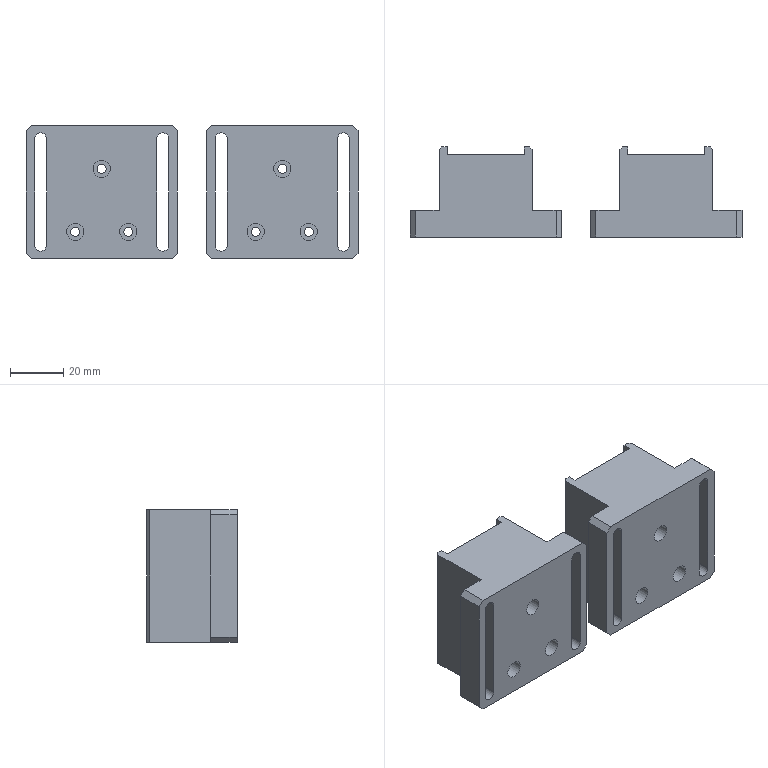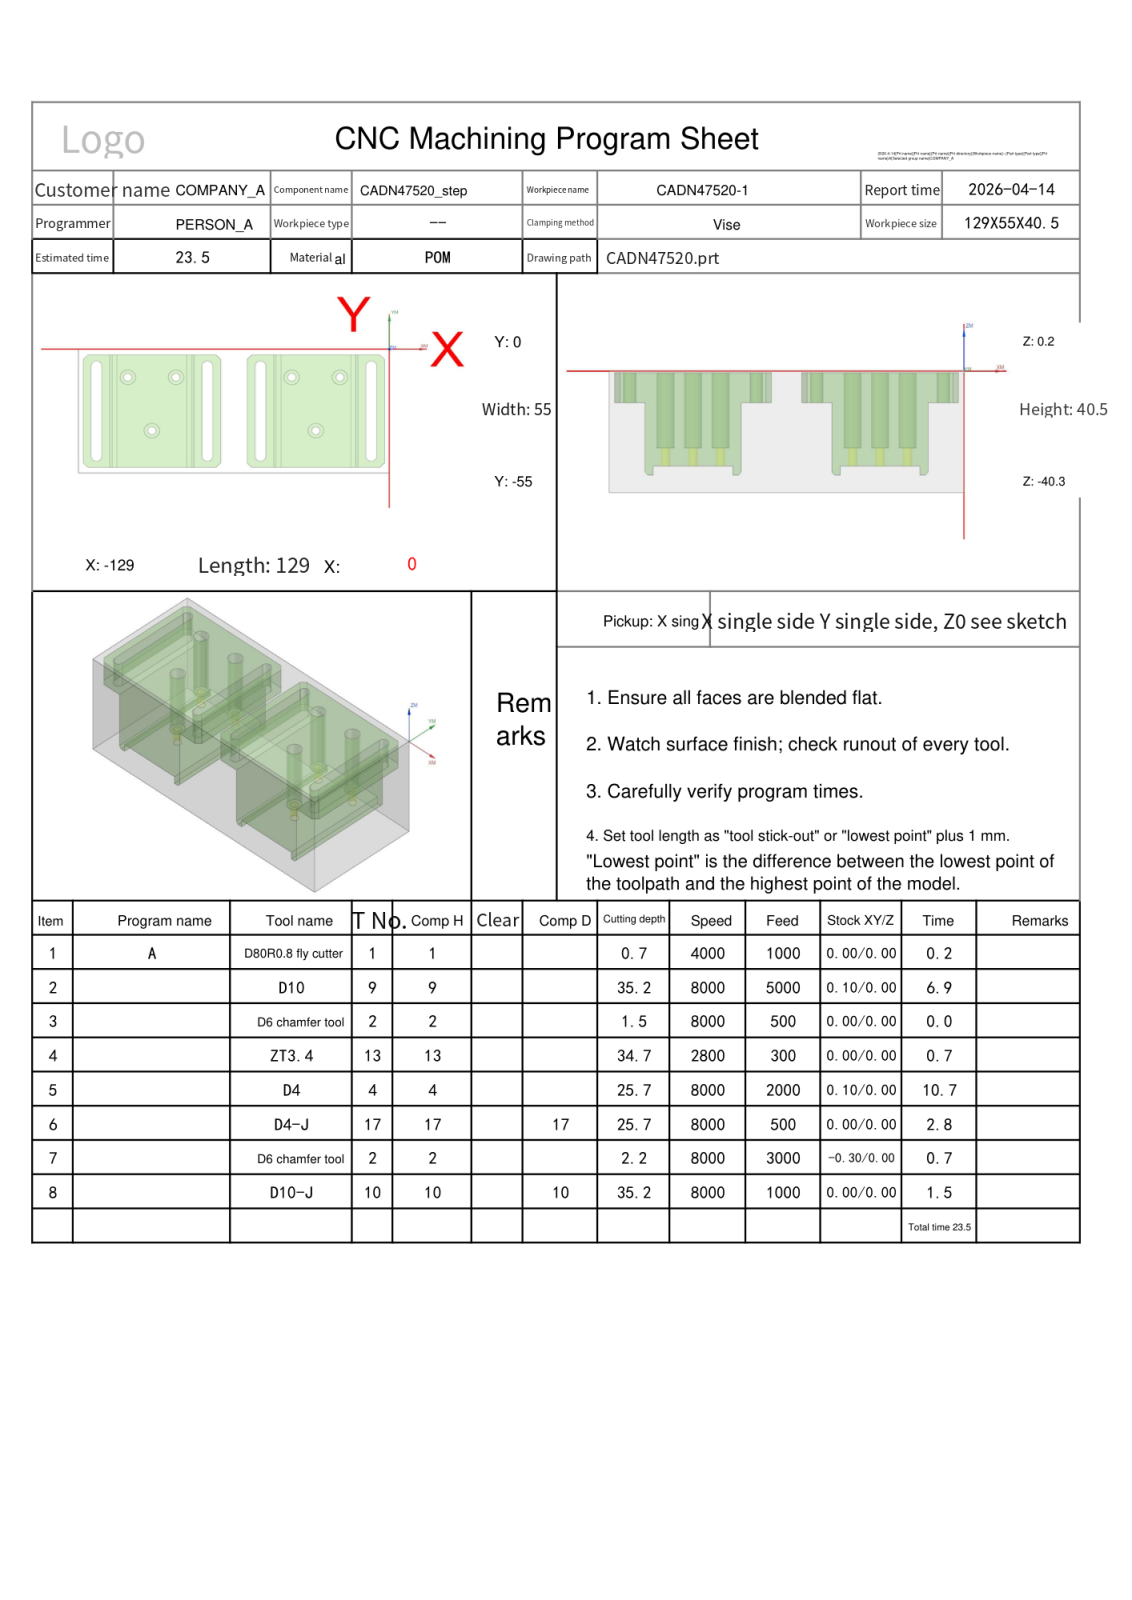NC program | NX | posted by the shop | part box 125 x 34 x 50 mm
Lines 34 to 772 of 5259:
N2 T09 M06
(D10  D=10. R=0. H=09 ce=0.10 di=0.00)
G00 G90 G54 X-98.5 Y-57.6 M03 S8000
G43 H09 Z19.5
M08
Z0.0
G01 X-125. Z-.055 F5000.
G02 X-128.606 Y-56.106 Z-.063 I0.0 J5.1
G01 X-130.606 Y-54.106 Z-.069
G02 X-132.1 Y-50.5 Z-.077 I3.606 J3.606
G01 Y-4.5 Z-.173
G02 X-130.606 Y-.894 Z-.181 I5.1 J0.0
G01 X-128.606 Y1.106 Z-.187
G02 X-125. Y2.6 Z-.195 I3.606 J-3.606
G01 X-72. Z-.305
G02 X-68.394 Y1.106 Z-.313 I0.0 J-5.1
G01 X-66.394 Y-.894 Z-.319
G02 X-64.9 Y-4.5 Z-.327 I-3.606 J-3.606
G01 Y-50.5 Z-.423
G02 X-66.394 Y-54.106 Z-.431 I-5.1 J0.0
G01 X-68.394 Y-56.106 Z-.437
G02 X-72. Y-57.6 Z-.445 I-3.606 J3.606
G01 X-125. Z-.555
G02 X-128.606 Y-56.106 Z-.563 I0.0 J5.1
G01 X-130.606 Y-54.106 Z-.569
G02 X-132.1 Y-50.5 Z-.577 I3.606 J3.606
G01 Y-4.5 Z-.673
G02 X-130.606 Y-.894 Z-.681 I5.1 J0.0
G01 X-128.606 Y1.106 Z-.687
G02 X-125. Y2.6 Z-.695 I3.606 J-3.606
G01 X-72. Z-.805
G02 X-68.394 Y1.106 Z-.813 I0.0 J-5.1
G01 X-66.394 Y-.894 Z-.819
G02 X-64.9 Y-4.5 Z-.827 I-3.606 J-3.606
G01 Y-50.5 Z-.923
G02 X-66.394 Y-54.106 Z-.931 I-5.1 J0.0
G01 X-68.394 Y-56.106 Z-.937
G02 X-72. Y-57.6 Z-.945 I-3.606 J3.606
G01 X-125. Z-1.055
G02 X-128.606 Y-56.106 Z-1.063 I0.0 J5.1
G01 X-130.606 Y-54.106 Z-1.069
G02 X-132.1 Y-50.5 Z-1.077 I3.606 J3.606
G01 Y-4.5 Z-1.173
G02 X-130.606 Y-.894 Z-1.181 I5.1 J0.0
G01 X-128.606 Y1.106 Z-1.187
G02 X-125. Y2.6 Z-1.195 I3.606 J-3.606
G01 X-72. Z-1.305
G02 X-68.394 Y1.106 Z-1.313 I0.0 J-5.1
G01 X-66.394 Y-.894 Z-1.319
G02 X-64.9 Y-4.5 Z-1.327 I-3.606 J-3.606
G01 Y-50.5 Z-1.423
G02 X-66.394 Y-54.106 Z-1.431 I-5.1 J0.0
G01 X-68.394 Y-56.106 Z-1.437
G02 X-72. Y-57.6 Z-1.445 I-3.606 J3.606
G01 X-125. Z-1.555
G02 X-128.606 Y-56.106 Z-1.563 I0.0 J5.1
G01 X-130.606 Y-54.106 Z-1.569
G02 X-132.1 Y-50.5 Z-1.577 I3.606 J3.606
G01 Y-4.5 Z-1.673
G02 X-130.606 Y-.894 Z-1.681 I5.1 J0.0
G01 X-128.606 Y1.106 Z-1.687
G02 X-125. Y2.6 Z-1.695 I3.606 J-3.606
G01 X-72. Z-1.805
G02 X-68.394 Y1.106 Z-1.813 I0.0 J-5.1
G01 X-66.394 Y-.894 Z-1.819
G02 X-64.9 Y-4.5 Z-1.827 I-3.606 J-3.606
G01 Y-50.5 Z-1.923
G02 X-66.394 Y-54.106 Z-1.931 I-5.1 J0.0
G01 X-68.394 Y-56.106 Z-1.937
G02 X-72. Y-57.6 Z-1.945 I-3.606 J3.606
G01 X-125. Z-2.055
G02 X-128.606 Y-56.106 Z-2.063 I0.0 J5.1
G01 X-130.606 Y-54.106 Z-2.069
G02 X-132.1 Y-50.5 Z-2.077 I3.606 J3.606
G01 Y-4.5 Z-2.173
G02 X-130.606 Y-.894 Z-2.181 I5.1 J0.0
G01 X-128.606 Y1.106 Z-2.187
G02 X-125. Y2.6 Z-2.195 I3.606 J-3.606
G01 X-72. Z-2.305
G02 X-68.394 Y1.106 Z-2.313 I0.0 J-5.1
G01 X-66.394 Y-.894 Z-2.319
G02 X-64.9 Y-4.5 Z-2.327 I-3.606 J-3.606
G01 Y-50.5 Z-2.423
G02 X-66.394 Y-54.106 Z-2.431 I-5.1 J0.0
G01 X-68.394 Y-56.106 Z-2.437
G02 X-72. Y-57.6 Z-2.445 I-3.606 J3.606
G01 X-125. Z-2.555
G02 X-128.606 Y-56.106 Z-2.563 I0.0 J5.1
G01 X-130.606 Y-54.106 Z-2.569
G02 X-132.1 Y-50.5 Z-2.577 I3.606 J3.606
G01 Y-4.5 Z-2.673
G02 X-130.606 Y-.894 Z-2.681 I5.1 J0.0
G01 X-128.606 Y1.106 Z-2.687
G02 X-125. Y2.6 Z-2.695 I3.606 J-3.606
G01 X-72. Z-2.805
G02 X-68.394 Y1.106 Z-2.813 I0.0 J-5.1
G01 X-66.394 Y-.894 Z-2.819
G02 X-64.9 Y-4.5 Z-2.827 I-3.606 J-3.606
G01 Y-50.5 Z-2.923
G02 X-66.394 Y-54.106 Z-2.931 I-5.1 J0.0
G01 X-68.394 Y-56.106 Z-2.937
G02 X-72. Y-57.6 Z-2.945 I-3.606 J3.606
G01 X-125. Z-3.055
G02 X-128.606 Y-56.106 Z-3.063 I0.0 J5.1
G01 X-130.606 Y-54.106 Z-3.069
G02 X-132.1 Y-50.5 Z-3.077 I3.606 J3.606
G01 Y-4.5 Z-3.173
G02 X-130.606 Y-.894 Z-3.181 I5.1 J0.0
G01 X-128.606 Y1.106 Z-3.187
G02 X-125. Y2.6 Z-3.195 I3.606 J-3.606
G01 X-72. Z-3.305
G02 X-68.394 Y1.106 Z-3.313 I0.0 J-5.1
G01 X-66.394 Y-.894 Z-3.319
G02 X-64.9 Y-4.5 Z-3.327 I-3.606 J-3.606
G01 Y-50.5 Z-3.423
G02 X-66.394 Y-54.106 Z-3.431 I-5.1 J0.0
G01 X-68.394 Y-56.106 Z-3.437
G02 X-72. Y-57.6 Z-3.445 I-3.606 J3.606
G01 X-125. Z-3.555
G02 X-128.606 Y-56.106 Z-3.563 I0.0 J5.1
G01 X-130.606 Y-54.106 Z-3.569
G02 X-132.1 Y-50.5 Z-3.577 I3.606 J3.606
G01 Y-4.5 Z-3.673
G02 X-130.606 Y-.894 Z-3.681 I5.1 J0.0
G01 X-128.606 Y1.106 Z-3.687
G02 X-125. Y2.6 Z-3.695 I3.606 J-3.606
G01 X-72. Z-3.805
G02 X-68.394 Y1.106 Z-3.813 I0.0 J-5.1
G01 X-66.394 Y-.894 Z-3.819
G02 X-64.9 Y-4.5 Z-3.827 I-3.606 J-3.606
G01 Y-50.5 Z-3.923
G02 X-66.394 Y-54.106 Z-3.931 I-5.1 J0.0
G01 X-68.394 Y-56.106 Z-3.937
G02 X-72. Y-57.6 Z-3.945 I-3.606 J3.606
G01 X-125. Z-4.055
G02 X-128.606 Y-56.106 Z-4.063 I0.0 J5.1
G01 X-130.606 Y-54.106 Z-4.069
G02 X-132.1 Y-50.5 Z-4.077 I3.606 J3.606
G01 Y-4.5 Z-4.173
G02 X-130.606 Y-.894 Z-4.181 I5.1 J0.0
G01 X-128.606 Y1.106 Z-4.187
G02 X-125. Y2.6 Z-4.195 I3.606 J-3.606
G01 X-72. Z-4.305
G02 X-68.394 Y1.106 Z-4.313 I0.0 J-5.1
G01 X-66.394 Y-.894 Z-4.319
G02 X-64.9 Y-4.5 Z-4.327 I-3.606 J-3.606
G01 Y-50.5 Z-4.423
G02 X-66.394 Y-54.106 Z-4.431 I-5.1 J0.0
G01 X-68.394 Y-56.106 Z-4.437
G02 X-72. Y-57.6 Z-4.445 I-3.606 J3.606
G01 X-125. Z-4.555
G02 X-128.606 Y-56.106 Z-4.563 I0.0 J5.1
G01 X-130.606 Y-54.106 Z-4.569
G02 X-132.1 Y-50.5 Z-4.577 I3.606 J3.606
G01 Y-4.5 Z-4.673
G02 X-130.606 Y-.894 Z-4.681 I5.1 J0.0
G01 X-128.606 Y1.106 Z-4.687
G02 X-125. Y2.6 Z-4.695 I3.606 J-3.606
G01 X-72. Z-4.805
G02 X-68.394 Y1.106 Z-4.813 I0.0 J-5.1
G01 X-66.394 Y-.894 Z-4.819
G02 X-64.9 Y-4.5 Z-4.827 I-3.606 J-3.606
G01 Y-50.5 Z-4.923
G02 X-66.394 Y-54.106 Z-4.931 I-5.1 J0.0
G01 X-68.394 Y-56.106 Z-4.937
G02 X-72. Y-57.6 Z-4.945 I-3.606 J3.606
G01 X-125. Z-5.055
G02 X-128.606 Y-56.106 Z-5.063 I0.0 J5.1
G01 X-130.606 Y-54.106 Z-5.069
G02 X-132.1 Y-50.5 Z-5.077 I3.606 J3.606
G01 Y-4.5 Z-5.173
G02 X-130.606 Y-.894 Z-5.181 I5.1 J0.0
G01 X-128.606 Y1.106 Z-5.187
G02 X-125. Y2.6 Z-5.195 I3.606 J-3.606
G01 X-72. Z-5.305
G02 X-68.394 Y1.106 Z-5.313 I0.0 J-5.1
G01 X-66.394 Y-.894 Z-5.319
G02 X-64.9 Y-4.5 Z-5.327 I-3.606 J-3.606
G01 Y-50.5 Z-5.423
G02 X-66.394 Y-54.106 Z-5.431 I-5.1 J0.0
G01 X-68.394 Y-56.106 Z-5.437
G02 X-72. Y-57.6 Z-5.445 I-3.606 J3.606
G01 X-125. Z-5.555
G02 X-128.606 Y-56.106 Z-5.563 I0.0 J5.1
G01 X-130.606 Y-54.106 Z-5.569
G02 X-132.1 Y-50.5 Z-5.577 I3.606 J3.606
G01 Y-4.5 Z-5.673
G02 X-130.606 Y-.894 Z-5.681 I5.1 J0.0
G01 X-128.606 Y1.106 Z-5.687
G02 X-125. Y2.6 Z-5.695 I3.606 J-3.606
G01 X-72. Z-5.805
G02 X-68.394 Y1.106 Z-5.813 I0.0 J-5.1
G01 X-66.394 Y-.894 Z-5.819
G02 X-64.9 Y-4.5 Z-5.827 I-3.606 J-3.606
G01 Y-50.5 Z-5.923
G02 X-66.394 Y-54.106 Z-5.931 I-5.1 J0.0
G01 X-68.394 Y-56.106 Z-5.937
G02 X-72. Y-57.6 Z-5.945 I-3.606 J3.606
G01 X-125. Z-6.055
G02 X-128.606 Y-56.106 Z-6.063 I0.0 J5.1
G01 X-130.606 Y-54.106 Z-6.069
G02 X-132.1 Y-50.5 Z-6.077 I3.606 J3.606
G01 Y-4.5 Z-6.173
G02 X-130.606 Y-.894 Z-6.181 I5.1 J0.0
G01 X-128.606 Y1.106 Z-6.187
G02 X-125. Y2.6 Z-6.195 I3.606 J-3.606
G01 X-72. Z-6.305
G02 X-68.394 Y1.106 Z-6.313 I0.0 J-5.1
G01 X-66.394 Y-.894 Z-6.319
G02 X-64.9 Y-4.5 Z-6.327 I-3.606 J-3.606
G01 Y-50.5 Z-6.423
G02 X-66.394 Y-54.106 Z-6.431 I-5.1 J0.0
G01 X-68.394 Y-56.106 Z-6.437
G02 X-72. Y-57.6 Z-6.445 I-3.606 J3.606
G01 X-125. Z-6.555
G02 X-128.606 Y-56.106 Z-6.563 I0.0 J5.1
G01 X-130.606 Y-54.106 Z-6.569
G02 X-132.1 Y-50.5 Z-6.577 I3.606 J3.606
G01 Y-4.5 Z-6.673
G02 X-130.606 Y-.894 Z-6.681 I5.1 J0.0
G01 X-128.606 Y1.106 Z-6.687
G02 X-125. Y2.6 Z-6.695 I3.606 J-3.606
G01 X-72. Z-6.805
G02 X-68.394 Y1.106 Z-6.813 I0.0 J-5.1
G01 X-66.394 Y-.894 Z-6.819
G02 X-64.9 Y-4.5 Z-6.827 I-3.606 J-3.606
G01 Y-50.5 Z-6.923
G02 X-66.394 Y-54.106 Z-6.931 I-5.1 J0.0
G01 X-68.394 Y-56.106 Z-6.937
G02 X-72. Y-57.6 Z-6.945 I-3.606 J3.606
G01 X-125. Z-7.055
G02 X-128.606 Y-56.106 Z-7.063 I0.0 J5.1
G01 X-130.606 Y-54.106 Z-7.069
G02 X-132.1 Y-50.5 Z-7.077 I3.606 J3.606
G01 Y-4.5 Z-7.173
G02 X-130.606 Y-.894 Z-7.181 I5.1 J0.0
G01 X-128.606 Y1.106 Z-7.187
G02 X-125. Y2.6 Z-7.195 I3.606 J-3.606
G01 X-72. Z-7.305
G02 X-68.394 Y1.106 Z-7.313 I0.0 J-5.1
G01 X-66.394 Y-.894 Z-7.319
G02 X-64.9 Y-4.5 Z-7.327 I-3.606 J-3.606
G01 Y-50.5 Z-7.423
G02 X-66.394 Y-54.106 Z-7.431 I-5.1 J0.0
G01 X-68.394 Y-56.106 Z-7.437
G02 X-72. Y-57.6 Z-7.445 I-3.606 J3.606
G01 X-125. Z-7.555
G02 X-128.606 Y-56.106 Z-7.563 I0.0 J5.1
G01 X-130.606 Y-54.106 Z-7.569
G02 X-132.1 Y-50.5 Z-7.577 I3.606 J3.606
G01 Y-4.5 Z-7.673
G02 X-130.606 Y-.894 Z-7.681 I5.1 J0.0
G01 X-128.606 Y1.106 Z-7.687
G02 X-125. Y2.6 Z-7.695 I3.606 J-3.606
G01 X-72. Z-7.805
G02 X-68.394 Y1.106 Z-7.813 I0.0 J-5.1
G01 X-66.394 Y-.894 Z-7.819
G02 X-64.9 Y-4.5 Z-7.827 I-3.606 J-3.606
G01 Y-50.5 Z-7.923
G02 X-66.394 Y-54.106 Z-7.931 I-5.1 J0.0
G01 X-68.394 Y-56.106 Z-7.937
G02 X-72. Y-57.6 Z-7.945 I-3.606 J3.606
G01 X-125. Z-8.055
G02 X-128.606 Y-56.106 Z-8.063 I0.0 J5.1
G01 X-130.606 Y-54.106 Z-8.069
G02 X-132.1 Y-50.5 Z-8.077 I3.606 J3.606
G01 Y-4.5 Z-8.173
G02 X-130.606 Y-.894 Z-8.181 I5.1 J0.0
G01 X-128.606 Y1.106 Z-8.187
G02 X-125. Y2.6 Z-8.195 I3.606 J-3.606
G01 X-72. Z-8.305
G02 X-68.394 Y1.106 Z-8.313 I0.0 J-5.1
G01 X-66.394 Y-.894 Z-8.319
G02 X-64.9 Y-4.5 Z-8.327 I-3.606 J-3.606
G01 Y-50.5 Z-8.423
G02 X-66.394 Y-54.106 Z-8.431 I-5.1 J0.0
G01 X-68.394 Y-56.106 Z-8.437
G02 X-72. Y-57.6 Z-8.445 I-3.606 J3.606
G01 X-125. Z-8.555
G02 X-128.606 Y-56.106 Z-8.563 I0.0 J5.1
G01 X-130.606 Y-54.106 Z-8.569
G02 X-132.1 Y-50.5 Z-8.577 I3.606 J3.606
G01 Y-4.5 Z-8.673
G02 X-130.606 Y-.894 Z-8.681 I5.1 J0.0
G01 X-128.606 Y1.106 Z-8.687
G02 X-125. Y2.6 Z-8.695 I3.606 J-3.606
G01 X-72. Z-8.805
G02 X-68.394 Y1.106 Z-8.813 I0.0 J-5.1
G01 X-66.394 Y-.894 Z-8.819
G02 X-64.9 Y-4.5 Z-8.827 I-3.606 J-3.606
G01 Y-50.5 Z-8.923
G02 X-66.394 Y-54.106 Z-8.931 I-5.1 J0.0
G01 X-68.394 Y-56.106 Z-8.937
G02 X-72. Y-57.6 Z-8.945 I-3.606 J3.606
G01 X-125. Z-9.055
G02 X-128.606 Y-56.106 Z-9.063 I0.0 J5.1
G01 X-130.606 Y-54.106 Z-9.069
G02 X-132.1 Y-50.5 Z-9.077 I3.606 J3.606
G01 Y-4.5 Z-9.173
G02 X-130.606 Y-.894 Z-9.181 I5.1 J0.0
G01 X-128.606 Y1.106 Z-9.187
G02 X-125. Y2.6 Z-9.195 I3.606 J-3.606
G01 X-72. Z-9.305
G02 X-68.394 Y1.106 Z-9.313 I0.0 J-5.1
G01 X-66.394 Y-.894 Z-9.319
G02 X-64.9 Y-4.5 Z-9.327 I-3.606 J-3.606
G01 Y-50.5 Z-9.423
G02 X-66.394 Y-54.106 Z-9.431 I-5.1 J0.0
G01 X-68.394 Y-56.106 Z-9.437
G02 X-72. Y-57.6 Z-9.445 I-3.606 J3.606
G01 X-125. Z-9.555
G02 X-128.606 Y-56.106 Z-9.563 I0.0 J5.1
G01 X-130.606 Y-54.106 Z-9.569
G02 X-132.1 Y-50.5 Z-9.577 I3.606 J3.606
G01 Y-4.5 Z-9.673
G02 X-130.606 Y-.894 Z-9.681 I5.1 J0.0
G01 X-128.606 Y1.106 Z-9.687
G02 X-125. Y2.6 Z-9.695 I3.606 J-3.606
G01 X-72. Z-9.805
G02 X-68.394 Y1.106 Z-9.813 I0.0 J-5.1
G01 X-66.394 Y-.894 Z-9.819
G02 X-64.9 Y-4.5 Z-9.827 I-3.606 J-3.606
G01 Y-50.5 Z-9.923
G02 X-66.394 Y-54.106 Z-9.931 I-5.1 J0.0
G01 X-68.394 Y-56.106 Z-9.937
G02 X-72. Y-57.6 Z-9.945 I-3.606 J3.606
G01 X-125. Z-10.055
G02 X-128.606 Y-56.106 Z-10.063 I0.0 J5.1
G01 X-130.606 Y-54.106 Z-10.069
G02 X-132.1 Y-50.5 Z-10.077 I3.606 J3.606
G01 Y-4.5 Z-10.173
G02 X-130.606 Y-.894 Z-10.181 I5.1 J0.0
G01 X-128.606 Y1.106 Z-10.187
G02 X-125. Y2.6 Z-10.195 I3.606 J-3.606
G01 X-72. Z-10.305
G02 X-68.394 Y1.106 Z-10.313 I0.0 J-5.1
G01 X-66.394 Y-.894 Z-10.319
G02 X-64.9 Y-4.5 Z-10.327 I-3.606 J-3.606
G01 Y-50.5 Z-10.423
G02 X-66.394 Y-54.106 Z-10.431 I-5.1 J0.0
G01 X-68.394 Y-56.106 Z-10.437
G02 X-72. Y-57.6 Z-10.445 I-3.606 J3.606
G01 X-125. Z-10.555
G02 X-128.606 Y-56.106 Z-10.563 I0.0 J5.1
G01 X-130.606 Y-54.106 Z-10.569
G02 X-132.1 Y-50.5 Z-10.577 I3.606 J3.606
G01 Y-4.5 Z-10.673
G02 X-130.606 Y-.894 Z-10.681 I5.1 J0.0
G01 X-128.606 Y1.106 Z-10.687
G02 X-125. Y2.6 Z-10.695 I3.606 J-3.606
G01 X-72. Z-10.805
G02 X-68.394 Y1.106 Z-10.813 I0.0 J-5.1
G01 X-66.394 Y-.894 Z-10.819
G02 X-64.9 Y-4.5 Z-10.827 I-3.606 J-3.606
G01 Y-50.5 Z-10.923
G02 X-66.394 Y-54.106 Z-10.931 I-5.1 J0.0
G01 X-68.394 Y-56.106 Z-10.937
G02 X-72. Y-57.6 Z-10.945 I-3.606 J3.606
G01 X-125. Z-11.055
G02 X-128.606 Y-56.106 Z-11.063 I0.0 J5.1
G01 X-130.606 Y-54.106 Z-11.069
G02 X-132.1 Y-50.5 Z-11.077 I3.606 J3.606
G01 Y-4.5 Z-11.173
G02 X-130.606 Y-.894 Z-11.181 I5.1 J0.0
G01 X-128.606 Y1.106 Z-11.187
G02 X-125. Y2.6 Z-11.195 I3.606 J-3.606
G01 X-72. Z-11.305
G02 X-68.394 Y1.106 Z-11.313 I0.0 J-5.1
G01 X-66.394 Y-.894 Z-11.319
G02 X-64.9 Y-4.5 Z-11.327 I-3.606 J-3.606
G01 Y-50.5 Z-11.423
G02 X-66.394 Y-54.106 Z-11.431 I-5.1 J0.0
G01 X-68.394 Y-56.106 Z-11.437
G02 X-72. Y-57.6 Z-11.445 I-3.606 J3.606
G01 X-125. Z-11.555
G02 X-128.606 Y-56.106 Z-11.563 I0.0 J5.1
G01 X-130.606 Y-54.106 Z-11.569
G02 X-132.1 Y-50.5 Z-11.577 I3.606 J3.606
G01 Y-4.5 Z-11.673
G02 X-130.606 Y-.894 Z-11.681 I5.1 J0.0
G01 X-128.606 Y1.106 Z-11.687
G02 X-125. Y2.6 Z-11.695 I3.606 J-3.606
G01 X-72. Z-11.805
G02 X-68.394 Y1.106 Z-11.813 I0.0 J-5.1
G01 X-66.394 Y-.894 Z-11.819
G02 X-64.9 Y-4.5 Z-11.827 I-3.606 J-3.606
G01 Y-50.5 Z-11.923
G02 X-66.394 Y-54.106 Z-11.931 I-5.1 J0.0
G01 X-68.394 Y-56.106 Z-11.937
G02 X-72. Y-57.6 Z-11.945 I-3.606 J3.606
G01 X-125. Z-12.055
G02 X-128.606 Y-56.106 Z-12.063 I0.0 J5.1
G01 X-130.606 Y-54.106 Z-12.069
G02 X-132.1 Y-50.5 Z-12.077 I3.606 J3.606
G01 Y-4.5 Z-12.173
G02 X-130.606 Y-.894 Z-12.181 I5.1 J0.0
G01 X-128.606 Y1.106 Z-12.187
G02 X-125. Y2.6 Z-12.195 I3.606 J-3.606
G01 X-72. Z-12.305
G02 X-68.394 Y1.106 Z-12.313 I0.0 J-5.1
G01 X-66.394 Y-.894 Z-12.319
G02 X-64.9 Y-4.5 Z-12.327 I-3.606 J-3.606
G01 Y-50.5 Z-12.423
G02 X-66.394 Y-54.106 Z-12.431 I-5.1 J0.0
G01 X-68.394 Y-56.106 Z-12.437
G02 X-72. Y-57.6 Z-12.445 I-3.606 J3.606
G01 X-125. Z-12.555
G02 X-128.606 Y-56.106 Z-12.563 I0.0 J5.1
G01 X-130.606 Y-54.106 Z-12.569
G02 X-132.1 Y-50.5 Z-12.577 I3.606 J3.606
G01 Y-4.5 Z-12.673
G02 X-130.606 Y-.894 Z-12.681 I5.1 J0.0
G01 X-128.606 Y1.106 Z-12.687
G02 X-125. Y2.6 Z-12.695 I3.606 J-3.606
G01 X-72. Z-12.805
G02 X-68.394 Y1.106 Z-12.813 I0.0 J-5.1
G01 X-66.394 Y-.894 Z-12.819
G02 X-64.9 Y-4.5 Z-12.827 I-3.606 J-3.606
G01 Y-50.5 Z-12.923
G02 X-66.394 Y-54.106 Z-12.931 I-5.1 J0.0
G01 X-68.394 Y-56.106 Z-12.937
G02 X-72. Y-57.6 Z-12.945 I-3.606 J3.606
G01 X-125. Z-13.055
G02 X-128.606 Y-56.106 Z-13.063 I0.0 J5.1
G01 X-130.606 Y-54.106 Z-13.069
G02 X-132.1 Y-50.5 Z-13.077 I3.606 J3.606
G01 Y-4.5 Z-13.173
G02 X-130.606 Y-.894 Z-13.181 I5.1 J0.0
G01 X-128.606 Y1.106 Z-13.187
G02 X-125. Y2.6 Z-13.195 I3.606 J-3.606
G01 X-72. Z-13.305
G02 X-68.394 Y1.106 Z-13.313 I0.0 J-5.1
G01 X-66.394 Y-.894 Z-13.319
G02 X-64.9 Y-4.5 Z-13.327 I-3.606 J-3.606
G01 Y-50.5 Z-13.423
G02 X-66.394 Y-54.106 Z-13.431 I-5.1 J0.0
G01 X-68.394 Y-56.106 Z-13.437
G02 X-72. Y-57.6 Z-13.445 I-3.606 J3.606
G01 X-125. Z-13.555
G02 X-128.606 Y-56.106 Z-13.563 I0.0 J5.1
G01 X-130.606 Y-54.106 Z-13.569
G02 X-132.1 Y-50.5 Z-13.577 I3.606 J3.606
G01 Y-4.5 Z-13.673
G02 X-130.606 Y-.894 Z-13.681 I5.1 J0.0
G01 X-128.606 Y1.106 Z-13.687
G02 X-125. Y2.6 Z-13.695 I3.606 J-3.606
G01 X-72. Z-13.805
G02 X-68.394 Y1.106 Z-13.813 I0.0 J-5.1
G01 X-66.394 Y-.894 Z-13.819
G02 X-64.9 Y-4.5 Z-13.827 I-3.606 J-3.606
G01 Y-50.5 Z-13.923
G02 X-66.394 Y-54.106 Z-13.931 I-5.1 J0.0
G01 X-68.394 Y-56.106 Z-13.937
G02 X-72. Y-57.6 Z-13.945 I-3.606 J3.606
G01 X-125. Z-14.055
G02 X-128.606 Y-56.106 Z-14.063 I0.0 J5.1
G01 X-130.606 Y-54.106 Z-14.069
G02 X-132.1 Y-50.5 Z-14.077 I3.606 J3.606
G01 Y-4.5 Z-14.173
G02 X-130.606 Y-.894 Z-14.181 I5.1 J0.0
G01 X-128.606 Y1.106 Z-14.187
G02 X-125. Y2.6 Z-14.195 I3.606 J-3.606
G01 X-72. Z-14.305
G02 X-68.394 Y1.106 Z-14.313 I0.0 J-5.1
G01 X-66.394 Y-.894 Z-14.319
G02 X-64.9 Y-4.5 Z-14.327 I-3.606 J-3.606
G01 Y-50.5 Z-14.423
G02 X-66.394 Y-54.106 Z-14.431 I-5.1 J0.0
G01 X-68.394 Y-56.106 Z-14.437
G02 X-72. Y-57.6 Z-14.445 I-3.606 J3.606
G01 X-125. Z-14.555
G02 X-128.606 Y-56.106 Z-14.563 I0.0 J5.1
G01 X-130.606 Y-54.106 Z-14.569
G02 X-132.1 Y-50.5 Z-14.577 I3.606 J3.606
G01 Y-4.5 Z-14.673
G02 X-130.606 Y-.894 Z-14.681 I5.1 J0.0
G01 X-128.606 Y1.106 Z-14.687
G02 X-125. Y2.6 Z-14.695 I3.606 J-3.606
G01 X-72. Z-14.805
G02 X-68.394 Y1.106 Z-14.813 I0.0 J-5.1
G01 X-66.394 Y-.894 Z-14.819
G02 X-64.9 Y-4.5 Z-14.827 I-3.606 J-3.606
G01 Y-50.5 Z-14.923
G02 X-66.394 Y-54.106 Z-14.931 I-5.1 J0.0
G01 X-68.394 Y-56.106 Z-14.937
G02 X-72. Y-57.6 Z-14.945 I-3.606 J3.606
G01 X-125. Z-15.055
G02 X-128.606 Y-56.106 Z-15.063 I0.0 J5.1
G01 X-130.606 Y-54.106 Z-15.069
G02 X-132.1 Y-50.5 Z-15.077 I3.606 J3.606
G01 Y-4.5 Z-15.173
G02 X-130.606 Y-.894 Z-15.181 I5.1 J0.0
G01 X-128.606 Y1.106 Z-15.187
G02 X-125. Y2.6 Z-15.195 I3.606 J-3.606
G01 X-72. Z-15.305
G02 X-68.394 Y1.106 Z-15.313 I0.0 J-5.1
G01 X-66.394 Y-.894 Z-15.319
G02 X-64.9 Y-4.5 Z-15.327 I-3.606 J-3.606
G01 Y-50.5 Z-15.423
G02 X-66.394 Y-54.106 Z-15.431 I-5.1 J0.0
G01 X-68.394 Y-56.106 Z-15.437
G02 X-72. Y-57.6 Z-15.445 I-3.606 J3.606
G01 X-125. Z-15.555
G02 X-128.606 Y-56.106 Z-15.563 I0.0 J5.1
G01 X-130.606 Y-54.106 Z-15.569
G02 X-132.1 Y-50.5 Z-15.577 I3.606 J3.606
G01 Y-4.5 Z-15.673
G02 X-130.606 Y-.894 Z-15.681 I5.1 J0.0
G01 X-128.606 Y1.106 Z-15.687
G02 X-125. Y2.6 Z-15.695 I3.606 J-3.606
G01 X-72. Z-15.805
G02 X-68.394 Y1.106 Z-15.813 I0.0 J-5.1
G01 X-66.394 Y-.894 Z-15.819
G02 X-64.9 Y-4.5 Z-15.827 I-3.606 J-3.606
G01 Y-50.5 Z-15.923
G02 X-66.394 Y-54.106 Z-15.931 I-5.1 J0.0
G01 X-68.394 Y-56.106 Z-15.937
G02 X-72. Y-57.6 Z-15.945 I-3.606 J3.606
G01 X-125. Z-16.055
G02 X-128.606 Y-56.106 Z-16.063 I0.0 J5.1
G01 X-130.606 Y-54.106 Z-16.069
G02 X-132.1 Y-50.5 Z-16.077 I3.606 J3.606
G01 Y-4.5 Z-16.173
G02 X-130.606 Y-.894 Z-16.181 I5.1 J0.0
G01 X-128.606 Y1.106 Z-16.187
G02 X-125. Y2.6 Z-16.195 I3.606 J-3.606
G01 X-72. Z-16.305
G02 X-68.394 Y1.106 Z-16.313 I0.0 J-5.1
G01 X-66.394 Y-.894 Z-16.319
G02 X-64.9 Y-4.5 Z-16.327 I-3.606 J-3.606
G01 Y-50.5 Z-16.423
G02 X-66.394 Y-54.106 Z-16.431 I-5.1 J0.0
G01 X-68.394 Y-56.106 Z-16.437
G02 X-72. Y-57.6 Z-16.445 I-3.606 J3.606
G01 X-125. Z-16.555
G02 X-128.606 Y-56.106 Z-16.563 I0.0 J5.1
G01 X-130.606 Y-54.106 Z-16.569
G02 X-132.1 Y-50.5 Z-16.577 I3.606 J3.606
G01 Y-4.5 Z-16.673
G02 X-130.606 Y-.894 Z-16.681 I5.1 J0.0
G01 X-128.606 Y1.106 Z-16.687
G02 X-125. Y2.6 Z-16.695 I3.606 J-3.606
G01 X-72. Z-16.805
G02 X-68.394 Y1.106 Z-16.813 I0.0 J-5.1
G01 X-66.394 Y-.894 Z-16.819
G02 X-64.9 Y-4.5 Z-16.827 I-3.606 J-3.606
G01 Y-50.5 Z-16.923
G02 X-66.394 Y-54.106 Z-16.931 I-5.1 J0.0
G01 X-68.394 Y-56.106 Z-16.937
G02 X-72. Y-57.6 Z-16.945 I-3.606 J3.606
G01 X-125. Z-17.055
G02 X-128.606 Y-56.106 Z-17.063 I0.0 J5.1
G01 X-130.606 Y-54.106 Z-17.069
G02 X-132.1 Y-50.5 Z-17.077 I3.606 J3.606
G01 Y-4.5 Z-17.173
G02 X-130.606 Y-.894 Z-17.181 I5.1 J0.0
G01 X-128.606 Y1.106 Z-17.187
G02 X-125. Y2.6 Z-17.195 I3.606 J-3.606
G01 X-72. Z-17.305
G02 X-68.394 Y1.106 Z-17.313 I0.0 J-5.1
G01 X-66.394 Y-.894 Z-17.319
G02 X-64.9 Y-4.5 Z-17.327 I-3.606 J-3.606
G01 Y-50.5 Z-17.423
G02 X-66.394 Y-54.106 Z-17.431 I-5.1 J0.0
G01 X-68.394 Y-56.106 Z-17.437
G02 X-72. Y-57.6 Z-17.445 I-3.606 J3.606
G01 X-125. Z-17.555
G02 X-128.606 Y-56.106 Z-17.563 I0.0 J5.1
G01 X-130.606 Y-54.106 Z-17.569
G02 X-132.1 Y-50.5 Z-17.577 I3.606 J3.606
G01 Y-4.5 Z-17.673
G02 X-130.606 Y-.894 Z-17.681 I5.1 J0.0
G01 X-128.606 Y1.106 Z-17.687
G02 X-125. Y2.6 Z-17.695 I3.606 J-3.606
G01 X-72. Z-17.805
G02 X-68.394 Y1.106 Z-17.813 I0.0 J-5.1
G01 X-66.394 Y-.894 Z-17.819
G02 X-64.9 Y-4.5 Z-17.827 I-3.606 J-3.606
G01 Y-50.5 Z-17.923
G02 X-66.394 Y-54.106 Z-17.931 I-5.1 J0.0
G01 X-68.394 Y-56.106 Z-17.937
G02 X-72. Y-57.6 Z-17.945 I-3.606 J3.606
G01 X-125. Z-18.055
G02 X-128.606 Y-56.106 Z-18.063 I0.0 J5.1
G01 X-130.606 Y-54.106 Z-18.069
G02 X-132.1 Y-50.5 Z-18.077 I3.606 J3.606
G01 Y-4.5 Z-18.173
G02 X-130.606 Y-.894 Z-18.181 I5.1 J0.0
G01 X-128.606 Y1.106 Z-18.187
G02 X-125. Y2.6 Z-18.195 I3.606 J-3.606
G01 X-72. Z-18.305
G02 X-68.394 Y1.106 Z-18.313 I0.0 J-5.1
G01 X-66.394 Y-.894 Z-18.319
G02 X-64.9 Y-4.5 Z-18.327 I-3.606 J-3.606
G01 Y-50.5 Z-18.423
G02 X-66.394 Y-54.106 Z-18.431 I-5.1 J0.0
G01 X-68.394 Y-56.106 Z-18.437
G02 X-72. Y-57.6 Z-18.445 I-3.606 J3.606
G01 X-125. Z-18.555
G02 X-128.606 Y-56.106 Z-18.563 I0.0 J5.1
G01 X-130.606 Y-54.106 Z-18.569
G02 X-132.1 Y-50.5 Z-18.577 I3.606 J3.606
G01 Y-4.5 Z-18.673
G02 X-130.606 Y-.894 Z-18.681 I5.1 J0.0
G01 X-128.606 Y1.106 Z-18.687
G02 X-125. Y2.6 Z-18.695 I3.606 J-3.606
G01 X-72. Z-18.805
G02 X-68.394 Y1.106 Z-18.813 I0.0 J-5.1
G01 X-66.394 Y-.894 Z-18.819
G02 X-64.9 Y-4.5 Z-18.827 I-3.606 J-3.606
G01 Y-50.5 Z-18.923
G02 X-66.394 Y-54.106 Z-18.931 I-5.1 J0.0
G01 X-68.394 Y-56.106 Z-18.937
G02 X-72. Y-57.6 Z-18.945 I-3.606 J3.606
G01 X-125. Z-19.055
G02 X-128.606 Y-56.106 Z-19.063 I0.0 J5.1
G01 X-130.606 Y-54.106 Z-19.069
G02 X-132.1 Y-50.5 Z-19.077 I3.606 J3.606
G01 Y-4.5 Z-19.173
G02 X-130.606 Y-.894 Z-19.181 I5.1 J0.0
G01 X-128.606 Y1.106 Z-19.187
G02 X-125. Y2.6 Z-19.195 I3.606 J-3.606
G01 X-72. Z-19.305
G02 X-68.394 Y1.106 Z-19.313 I0.0 J-5.1
G01 X-66.394 Y-.894 Z-19.319
G02 X-64.9 Y-4.5 Z-19.327 I-3.606 J-3.606
G01 Y-50.5 Z-19.423
G02 X-66.394 Y-54.106 Z-19.431 I-5.1 J0.0
G01 X-68.394 Y-56.106 Z-19.437
G02 X-72. Y-57.6 Z-19.445 I-3.606 J3.606
G01 X-125. Z-19.555
G02 X-128.606 Y-56.106 Z-19.563 I0.0 J5.1
G01 X-130.606 Y-54.106 Z-19.569
G02 X-132.1 Y-50.5 Z-19.577 I3.606 J3.606
G01 Y-4.5 Z-19.673
G02 X-130.606 Y-.894 Z-19.681 I5.1 J0.0
G01 X-128.606 Y1.106 Z-19.687
G02 X-125. Y2.6 Z-19.695 I3.606 J-3.606
G01 X-72. Z-19.805
G02 X-68.394 Y1.106 Z-19.813 I0.0 J-5.1
G01 X-66.394 Y-.894 Z-19.819
G02 X-64.9 Y-4.5 Z-19.827 I-3.606 J-3.606
G01 Y-50.5 Z-19.923
G02 X-66.394 Y-54.106 Z-19.931 I-5.1 J0.0
G01 X-68.394 Y-56.106 Z-19.937
G02 X-72. Y-57.6 Z-19.945 I-3.606 J3.606
G01 X-125. Z-20.055
G02 X-128.606 Y-56.106 Z-20.063 I0.0 J5.1
G01 X-130.606 Y-54.106 Z-20.069
G02 X-132.1 Y-50.5 Z-20.077 I3.606 J3.606
G01 Y-4.5 Z-20.173
G02 X-130.606 Y-.894 Z-20.181 I5.1 J0.0
G01 X-128.606 Y1.106 Z-20.187
G02 X-125. Y2.6 Z-20.195 I3.606 J-3.606
G01 X-72. Z-20.305
G02 X-68.394 Y1.106 Z-20.313 I0.0 J-5.1
G01 X-66.394 Y-.894 Z-20.319
G02 X-64.9 Y-4.5 Z-20.327 I-3.606 J-3.606
G01 Y-50.5 Z-20.423
G02 X-66.394 Y-54.106 Z-20.431 I-5.1 J0.0
G01 X-68.394 Y-56.106 Z-20.437
G02 X-72. Y-57.6 Z-20.445 I-3.606 J3.606
G01 X-125. Z-20.555
G02 X-128.606 Y-56.106 Z-20.563 I0.0 J5.1
G01 X-130.606 Y-54.106 Z-20.569
G02 X-132.1 Y-50.5 Z-20.577 I3.606 J3.606
G01 Y-4.5 Z-20.673
G02 X-130.606 Y-.894 Z-20.681 I5.1 J0.0
G01 X-128.606 Y1.106 Z-20.687
G02 X-125. Y2.6 Z-20.695 I3.606 J-3.606
G01 X-72. Z-20.805
G02 X-68.394 Y1.106 Z-20.813 I0.0 J-5.1
G01 X-66.394 Y-.894 Z-20.819
G02 X-64.9 Y-4.5 Z-20.827 I-3.606 J-3.606
G01 Y-50.5 Z-20.923
G02 X-66.394 Y-54.106 Z-20.931 I-5.1 J0.0
G01 X-68.394 Y-56.106 Z-20.937
G02 X-72. Y-57.6 Z-20.945 I-3.606 J3.606
G01 X-125. Z-21.055
G02 X-128.606 Y-56.106 Z-21.063 I0.0 J5.1
G01 X-130.606 Y-54.106 Z-21.069
G02 X-132.1 Y-50.5 Z-21.077 I3.606 J3.606
G01 Y-4.5 Z-21.173
G02 X-130.606 Y-.894 Z-21.181 I5.1 J0.0
G01 X-128.606 Y1.106 Z-21.187
G02 X-125. Y2.6 Z-21.195 I3.606 J-3.606
G01 X-72. Z-21.305
G02 X-68.394 Y1.106 Z-21.313 I0.0 J-5.1
G01 X-66.394 Y-.894 Z-21.319
G02 X-64.9 Y-4.5 Z-21.327 I-3.606 J-3.606
G01 Y-50.5 Z-21.423
G02 X-66.394 Y-54.106 Z-21.431 I-5.1 J0.0
G01 X-68.394 Y-56.106 Z-21.437
G02 X-72. Y-57.6 Z-21.445 I-3.606 J3.606
G01 X-125. Z-21.555
G02 X-128.606 Y-56.106 Z-21.563 I0.0 J5.1
G01 X-130.606 Y-54.106 Z-21.569
G02 X-132.1 Y-50.5 Z-21.577 I3.606 J3.606
G01 Y-4.5 Z-21.673
G02 X-130.606 Y-.894 Z-21.681 I5.1 J0.0
G01 X-128.606 Y1.106 Z-21.687
G02 X-125. Y2.6 Z-21.695 I3.606 J-3.606
G01 X-72. Z-21.805
G02 X-68.394 Y1.106 Z-21.813 I0.0 J-5.1
G01 X-66.394 Y-.894 Z-21.819
G02 X-64.9 Y-4.5 Z-21.827 I-3.606 J-3.606
G01 Y-50.5 Z-21.923
G02 X-66.394 Y-54.106 Z-21.931 I-5.1 J0.0
G01 X-68.394 Y-56.106 Z-21.937
G02 X-72. Y-57.6 Z-21.945 I-3.606 J3.606
G01 X-125. Z-22.055
G02 X-128.606 Y-56.106 Z-22.063 I0.0 J5.1
G01 X-130.606 Y-54.106 Z-22.069
G02 X-132.1 Y-50.5 Z-22.077 I3.606 J3.606
G01 Y-4.5 Z-22.173
G02 X-130.606 Y-.894 Z-22.181 I5.1 J0.0
G01 X-128.606 Y1.106 Z-22.187
G02 X-125. Y2.6 Z-22.195 I3.606 J-3.606
G01 X-72. Z-22.305
G02 X-68.394 Y1.106 Z-22.313 I0.0 J-5.1
G01 X-66.394 Y-.894 Z-22.319
G02 X-64.9 Y-4.5 Z-22.327 I-3.606 J-3.606
G01 Y-50.5 Z-22.423
G02 X-66.394 Y-54.106 Z-22.431 I-5.1 J0.0
G01 X-68.394 Y-56.106 Z-22.437
G02 X-72. Y-57.6 Z-22.445 I-3.606 J3.606
G01 X-125. Z-22.555
G02 X-128.606 Y-56.106 Z-22.563 I0.0 J5.1
G01 X-130.606 Y-54.106 Z-22.569
G02 X-132.1 Y-50.5 Z-22.577 I3.606 J3.606
G01 Y-4.5 Z-22.673
G02 X-130.606 Y-.894 Z-22.681 I5.1 J0.0
G01 X-128.606 Y1.106 Z-22.687
G02 X-125. Y2.6 Z-22.695 I3.606 J-3.606
G01 X-72. Z-22.805
G02 X-68.394 Y1.106 Z-22.813 I0.0 J-5.1
G01 X-66.394 Y-.894 Z-22.819
G02 X-64.9 Y-4.5 Z-22.827 I-3.606 J-3.606
G01 Y-50.5 Z-22.923